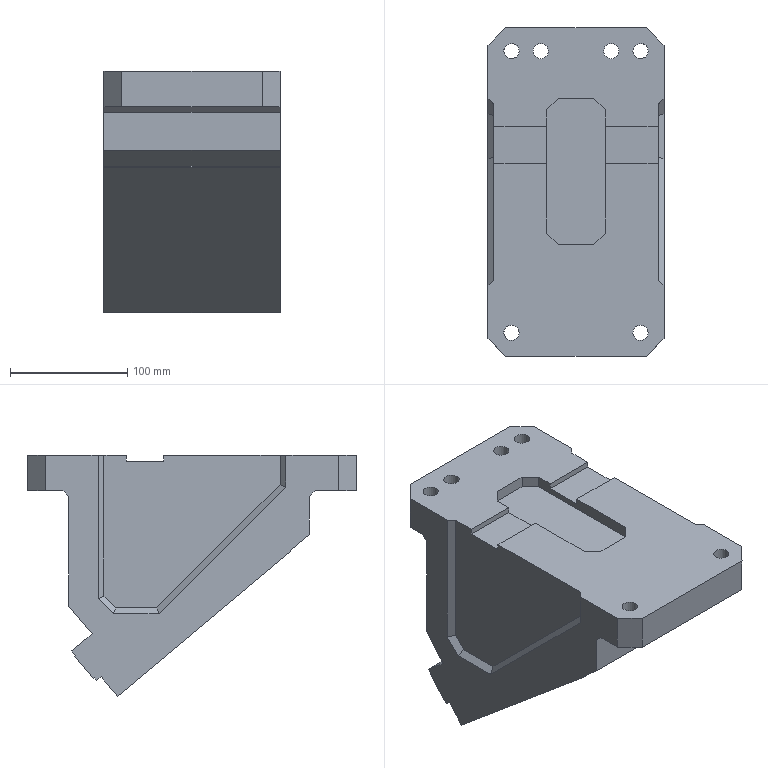Part | NX | features solid 2 | 1 solid | 69 faces | box 150 x 280 x 205.536 mm | volume 4538120 mm3 | plane 59 | cylinder 10 | commonest cylinder face diameters 13 x6 20 x4